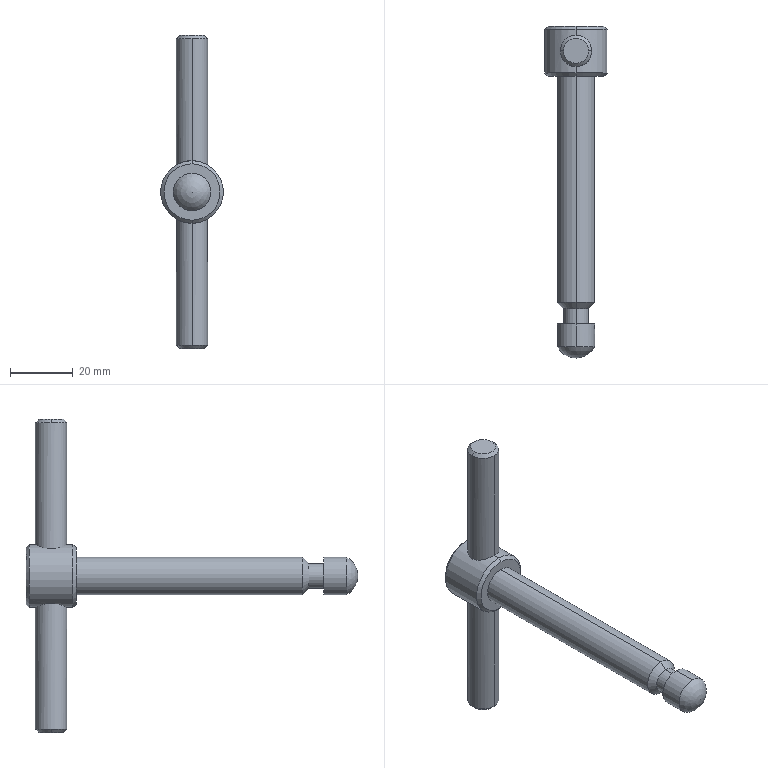Part | SolidWorks | features Revolution 5, Chamfer 4, Dome 3 | 1 solid | 28 faces | box 20 x 106 x 100 mm | volume 20892 mm3 | cylinder 12 | cone 10 | plane 5 | sphere 1 | commonest cylinder face diameters 10 x4 12 x4 7.92 x2 20 x2
STEP:
#1=CARTESIAN_POINT('',(0.,-90.304,-3.96));
#2=VERTEX_POINT('',#1);
#3=CARTESIAN_POINT('',(0.,-90.304,3.96));
#4=VERTEX_POINT('',#3);
#5=CARTESIAN_POINT('',(0.,-90.304,0.));
#6=DIRECTION('',(0.,-1.,0.));
#7=DIRECTION('',(0.,0.,1.));
#8=AXIS2_PLACEMENT_3D('',#5,#6,#7);
#9=CIRCLE('',#8,3.96);
#10=EDGE_CURVE('',#2,#4,#9,.T.);
#11=ORIENTED_EDGE('',*,*,#10,.F.);
#12=CARTESIAN_POINT('',(0.,-88.264,-6.));
#13=VERTEX_POINT('',#12);
#14=CARTESIAN_POINT('',(0.,-88.264,-6.));
#15=DIRECTION('',(0.,0.7071,-0.7071));
#16=VECTOR('',#15,1000.);
#17=LINE('',#14,#16);
#18=EDGE_CURVE('',#2,#13,#17,.T.);
#19=ORIENTED_EDGE('',*,*,#18,.T.);
#20=CARTESIAN_POINT('',(0.,-88.264,6.));
#21=VERTEX_POINT('',#20);
#22=CARTESIAN_POINT('',(0.,-88.264,0.));
#23=DIRECTION('',(0.,1.,0.));
#24=DIRECTION('',(0.,0.,1.));
#25=AXIS2_PLACEMENT_3D('',#22,#23,#24);
#26=CIRCLE('',#25,6.);
#27=EDGE_CURVE('',#21,#13,#26,.T.);
#28=ORIENTED_EDGE('',*,*,#27,.F.);
#29=CARTESIAN_POINT('',(0.,-88.264,6.));
#30=DIRECTION('',(0.,0.7071,0.7071));
#31=VECTOR('',#30,1000.);
#32=LINE('',#29,#31);
#33=EDGE_CURVE('',#4,#21,#32,.T.);
#34=ORIENTED_EDGE('',*,*,#33,.F.);
#35=EDGE_LOOP('',(#11,#19,#28,#34));
#36=FACE_OUTER_BOUND('',#35,.T.);
#37=CARTESIAN_POINT('',(0.,-88.264,0.));
#38=DIRECTION('',(0.,1.,0.));
#39=DIRECTION('',(0.,0.,1.));
#40=AXIS2_PLACEMENT_3D('',#37,#38,#39);
#41=CONICAL_SURFACE('',#40,6.,0.7854);
#42=ADVANCED_FACE('',(#36),#41,.T.);
#43=CARTESIAN_POINT('',(0.,-102.4,6.));
#44=VERTEX_POINT('',#43);
#45=CARTESIAN_POINT('',(0.,-102.4,-6.));
#46=VERTEX_POINT('',#45);
#47=CARTESIAN_POINT('',(0.,-102.4,0.));
#48=DIRECTION('',(0.,1.,0.));
#49=DIRECTION('',(0.,0.,1.));
#50=AXIS2_PLACEMENT_3D('',#47,#48,#49);
#51=CIRCLE('',#50,6.);
#52=EDGE_CURVE('',#44,#46,#51,.T.);
#53=ORIENTED_EDGE('',*,*,#52,.T.);
#54=CARTESIAN_POINT('',(0.,-95.142,-6.));
#55=VERTEX_POINT('',#54);
#56=CARTESIAN_POINT('',(0.,25.503,-6.));
#57=DIRECTION('',(0.,1.,0.));
#58=VECTOR('',#57,1000.);
#59=LINE('',#56,#58);
#60=EDGE_CURVE('',#46,#55,#59,.T.);
#61=ORIENTED_EDGE('',*,*,#60,.T.);
#62=CARTESIAN_POINT('',(0.,-95.142,6.));
#63=VERTEX_POINT('',#62);
#64=CARTESIAN_POINT('',(0.,-95.142,0.));
#65=DIRECTION('',(0.,1.,0.));
#66=DIRECTION('',(0.,0.,1.));
#67=AXIS2_PLACEMENT_3D('',#64,#65,#66);
#68=CIRCLE('',#67,6.);
#69=EDGE_CURVE('',#63,#55,#68,.T.);
#70=ORIENTED_EDGE('',*,*,#69,.F.);
#71=CARTESIAN_POINT('',(0.,25.503,6.));
#72=DIRECTION('',(0.,1.,0.));
#73=VECTOR('',#72,1000.);
#74=LINE('',#71,#73);
#75=EDGE_CURVE('',#44,#63,#74,.T.);
#76=ORIENTED_EDGE('',*,*,#75,.F.);
#77=EDGE_LOOP('',(#53,#61,#70,#76));
#78=FACE_OUTER_BOUND('',#77,.T.);
#79=CARTESIAN_POINT('',(0.,25.503,0.));
#80=DIRECTION('',(0.,1.,0.));
#81=DIRECTION('',(0.,0.,1.));
#82=AXIS2_PLACEMENT_3D('',#79,#80,#81);
#83=CYLINDRICAL_SURFACE('',#82,6.);
#84=ADVANCED_FACE('',(#78),#83,.T.);
#85=CARTESIAN_POINT('',(0.,-95.142,3.96));
#86=VERTEX_POINT('',#85);
#87=CARTESIAN_POINT('',(0.,-95.142,-3.96));
#88=VERTEX_POINT('',#87);
#89=CARTESIAN_POINT('',(0.,-95.142,0.));
#90=DIRECTION('',(0.,1.,0.));
#91=DIRECTION('',(0.,0.,1.));
#92=AXIS2_PLACEMENT_3D('',#89,#90,#91);
#93=CIRCLE('',#92,3.96);
#94=EDGE_CURVE('',#86,#88,#93,.T.);
#95=ORIENTED_EDGE('',*,*,#94,.T.);
#96=CARTESIAN_POINT('',(0.,25.503,-3.96));
#97=DIRECTION('',(0.,1.,0.));
#98=VECTOR('',#97,1000.);
#99=LINE('',#96,#98);
#100=EDGE_CURVE('',#88,#2,#99,.T.);
#101=ORIENTED_EDGE('',*,*,#100,.T.);
#102=ORIENTED_EDGE('',*,*,#10,.T.);
#103=CARTESIAN_POINT('',(0.,25.503,3.96));
#104=DIRECTION('',(0.,1.,0.));
#105=VECTOR('',#104,1000.);
#106=LINE('',#103,#105);
#107=EDGE_CURVE('',#86,#4,#106,.T.);
#108=ORIENTED_EDGE('',*,*,#107,.F.);
#109=EDGE_LOOP('',(#95,#101,#102,#108));
#110=FACE_OUTER_BOUND('',#109,.T.);
#111=CARTESIAN_POINT('',(0.,25.503,0.));
#112=DIRECTION('',(0.,1.,0.));
#113=DIRECTION('',(0.,0.,1.));
#114=AXIS2_PLACEMENT_3D('',#111,#112,#113);
#115=CYLINDRICAL_SURFACE('',#114,3.96);
#116=ADVANCED_FACE('',(#110),#115,.T.);
#117=CARTESIAN_POINT('',(0.,0.,9.));
#118=VERTEX_POINT('',#117);
#119=CARTESIAN_POINT('',(0.,0.,-9.));
#120=VERTEX_POINT('',#119);
#121=CARTESIAN_POINT('',(0.,0.,0.));
#122=DIRECTION('',(0.,1.,0.));
#123=DIRECTION('',(0.,0.,-1.));
#124=AXIS2_PLACEMENT_3D('',#121,#122,#123);
#125=CIRCLE('',#124,9.);
#126=EDGE_CURVE('',#118,#120,#125,.T.);
#127=ORIENTED_EDGE('',*,*,#126,.F.);
#128=CARTESIAN_POINT('',(0.,-1.,10.));
#129=VERTEX_POINT('',#128);
#130=CARTESIAN_POINT('',(0.,0.,9.));
#131=DIRECTION('',(0.,-0.7071,0.7071));
#132=VECTOR('',#131,1000.);
#133=LINE('',#130,#132);
#134=EDGE_CURVE('',#118,#129,#133,.T.);
#135=ORIENTED_EDGE('',*,*,#134,.T.);
#136=CARTESIAN_POINT('',(0.,-1.,-10.));
#137=VERTEX_POINT('',#136);
#138=CARTESIAN_POINT('',(0.,-1.,0.));
#139=DIRECTION('',(0.,-1.,0.));
#140=DIRECTION('',(0.,0.,-1.));
#141=AXIS2_PLACEMENT_3D('',#138,#139,#140);
#142=CIRCLE('',#141,10.);
#143=EDGE_CURVE('',#137,#129,#142,.T.);
#144=ORIENTED_EDGE('',*,*,#143,.F.);
#145=CARTESIAN_POINT('',(0.,0.,-9.));
#146=DIRECTION('',(0.,-0.7071,-0.7071));
#147=VECTOR('',#146,1000.);
#148=LINE('',#145,#147);
#149=EDGE_CURVE('',#120,#137,#148,.T.);
#150=ORIENTED_EDGE('',*,*,#149,.F.);
#151=EDGE_LOOP('',(#127,#135,#144,#150));
#152=FACE_OUTER_BOUND('',#151,.T.);
#153=CARTESIAN_POINT('',(0.,0.,0.));
#154=DIRECTION('',(0.,-1.,0.));
#155=DIRECTION('',(0.,0.,-1.));
#156=AXIS2_PLACEMENT_3D('',#153,#154,#155);
#157=CONICAL_SURFACE('',#156,9.,0.7854);
#158=ADVANCED_FACE('',(#152),#157,.T.);
#159=CARTESIAN_POINT('',(0.,-16.,-9.));
#160=VERTEX_POINT('',#159);
#161=CARTESIAN_POINT('',(0.,-16.,9.));
#162=VERTEX_POINT('',#161);
#163=CARTESIAN_POINT('',(0.,-16.,0.));
#164=DIRECTION('',(0.,-1.,0.));
#165=DIRECTION('',(0.,0.,1.));
#166=AXIS2_PLACEMENT_3D('',#163,#164,#165);
#167=CIRCLE('',#166,9.);
#168=EDGE_CURVE('',#160,#162,#167,.T.);
#169=ORIENTED_EDGE('',*,*,#168,.F.);
#170=CARTESIAN_POINT('',(0.,-15.,-10.));
#171=VERTEX_POINT('',#170);
#172=CARTESIAN_POINT('',(0.,-15.,-10.));
#173=DIRECTION('',(0.,0.7071,-0.7071));
#174=VECTOR('',#173,1000.);
#175=LINE('',#172,#174);
#176=EDGE_CURVE('',#160,#171,#175,.T.);
#177=ORIENTED_EDGE('',*,*,#176,.T.);
#178=CARTESIAN_POINT('',(0.,-15.,10.));
#179=VERTEX_POINT('',#178);
#180=CARTESIAN_POINT('',(0.,-15.,0.));
#181=DIRECTION('',(0.,1.,0.));
#182=DIRECTION('',(0.,0.,1.));
#183=AXIS2_PLACEMENT_3D('',#180,#181,#182);
#184=CIRCLE('',#183,10.);
#185=EDGE_CURVE('',#179,#171,#184,.T.);
#186=ORIENTED_EDGE('',*,*,#185,.F.);
#187=CARTESIAN_POINT('',(0.,-15.,10.));
#188=DIRECTION('',(0.,0.7071,0.7071));
#189=VECTOR('',#188,1000.);
#190=LINE('',#187,#189);
#191=EDGE_CURVE('',#162,#179,#190,.T.);
#192=ORIENTED_EDGE('',*,*,#191,.F.);
#193=EDGE_LOOP('',(#169,#177,#186,#192));
#194=FACE_OUTER_BOUND('',#193,.T.);
#195=CARTESIAN_POINT('',(0.,-15.,0.));
#196=DIRECTION('',(0.,1.,0.));
#197=DIRECTION('',(0.,0.,1.));
#198=AXIS2_PLACEMENT_3D('',#195,#196,#197);
#199=CONICAL_SURFACE('',#198,10.,0.7854);
#200=ADVANCED_FACE('',(#194),#199,.T.);
#201=CARTESIAN_POINT('',(4.,-8.,50.));
#202=VERTEX_POINT('',#201);
#203=CARTESIAN_POINT('',(-4.,-8.,50.));
#204=VERTEX_POINT('',#203);
#205=CARTESIAN_POINT('',(0.,-8.,50.));
#206=DIRECTION('',(0.,0.,1.));
#207=DIRECTION('',(0.,-1.,0.));
#208=AXIS2_PLACEMENT_3D('',#205,#206,#207);
#209=CIRCLE('',#208,4.);
#210=EDGE_CURVE('',#202,#204,#209,.T.);
#211=ORIENTED_EDGE('',*,*,#210,.F.);
#212=CARTESIAN_POINT('',(5.,-8.,49.));
#213=VERTEX_POINT('',#212);
#214=CARTESIAN_POINT('',(5.,-8.,49.));
#215=DIRECTION('',(0.7071,0.,-0.7071));
#216=VECTOR('',#215,1000.);
#217=LINE('',#214,#216);
#218=EDGE_CURVE('',#202,#213,#217,.T.);
#219=ORIENTED_EDGE('',*,*,#218,.T.);
#220=CARTESIAN_POINT('',(0.,-3.,49.));
#221=VERTEX_POINT('',#220);
#222=CARTESIAN_POINT('',(0.,-8.,49.));
#223=DIRECTION('',(0.,0.,-1.));
#224=DIRECTION('',(1.,0.,0.));
#225=AXIS2_PLACEMENT_3D('',#222,#223,#224);
#226=CIRCLE('',#225,5.);
#227=EDGE_CURVE('',#221,#213,#226,.T.);
#228=ORIENTED_EDGE('',*,*,#227,.F.);
#229=CARTESIAN_POINT('',(-5.,-8.,49.));
#230=VERTEX_POINT('',#229);
#231=CARTESIAN_POINT('',(0.,-8.,49.));
#232=DIRECTION('',(0.,0.,-1.));
#233=DIRECTION('',(1.,0.,0.));
#234=AXIS2_PLACEMENT_3D('',#231,#232,#233);
#235=CIRCLE('',#234,5.);
#236=EDGE_CURVE('',#230,#221,#235,.T.);
#237=ORIENTED_EDGE('',*,*,#236,.F.);
#238=CARTESIAN_POINT('',(-5.,-8.,49.));
#239=DIRECTION('',(-0.7071,0.,-0.7071));
#240=VECTOR('',#239,1000.);
#241=LINE('',#238,#240);
#242=EDGE_CURVE('',#204,#230,#241,.T.);
#243=ORIENTED_EDGE('',*,*,#242,.F.);
#244=EDGE_LOOP('',(#211,#219,#228,#237,#243));
#245=FACE_OUTER_BOUND('',#244,.T.);
#246=CARTESIAN_POINT('',(0.,-8.,49.));
#247=DIRECTION('',(0.,0.,-1.));
#248=DIRECTION('',(-1.,0.,0.));
#249=AXIS2_PLACEMENT_3D('',#246,#247,#248);
#250=CONICAL_SURFACE('',#249,5.,0.7854);
#251=ADVANCED_FACE('',(#245),#250,.T.);
#252=CARTESIAN_POINT('',(-4.,-8.,-50.));
#253=VERTEX_POINT('',#252);
#254=CARTESIAN_POINT('',(4.,-8.,-50.));
#255=VERTEX_POINT('',#254);
#256=CARTESIAN_POINT('',(0.,-8.,-50.));
#257=DIRECTION('',(0.,0.,-1.));
#258=DIRECTION('',(0.,1.,0.));
#259=AXIS2_PLACEMENT_3D('',#256,#257,#258);
#260=CIRCLE('',#259,4.);
#261=EDGE_CURVE('',#253,#255,#260,.T.);
#262=ORIENTED_EDGE('',*,*,#261,.F.);
#263=CARTESIAN_POINT('',(-5.,-8.,-49.));
#264=VERTEX_POINT('',#263);
#265=CARTESIAN_POINT('',(-4.,-8.,-50.));
#266=DIRECTION('',(-0.7071,0.,0.7071));
#267=VECTOR('',#266,1000.);
#268=LINE('',#265,#267);
#269=EDGE_CURVE('',#253,#264,#268,.T.);
#270=ORIENTED_EDGE('',*,*,#269,.T.);
#271=CARTESIAN_POINT('',(0.,-3.,-49.));
#272=VERTEX_POINT('',#271);
#273=CARTESIAN_POINT('',(0.,-8.,-49.));
#274=DIRECTION('',(0.,0.,1.));
#275=DIRECTION('',(-1.,0.,0.));
#276=AXIS2_PLACEMENT_3D('',#273,#274,#275);
#277=CIRCLE('',#276,5.);
#278=EDGE_CURVE('',#272,#264,#277,.T.);
#279=ORIENTED_EDGE('',*,*,#278,.F.);
#280=CARTESIAN_POINT('',(5.,-8.,-49.));
#281=VERTEX_POINT('',#280);
#282=CARTESIAN_POINT('',(0.,-8.,-49.));
#283=DIRECTION('',(0.,0.,1.));
#284=DIRECTION('',(-1.,0.,0.));
#285=AXIS2_PLACEMENT_3D('',#282,#283,#284);
#286=CIRCLE('',#285,5.);
#287=EDGE_CURVE('',#281,#272,#286,.T.);
#288=ORIENTED_EDGE('',*,*,#287,.F.);
#289=CARTESIAN_POINT('',(4.,-8.,-50.));
#290=DIRECTION('',(0.7071,0.,0.7071));
#291=VECTOR('',#290,1000.);
#292=LINE('',#289,#291);
#293=EDGE_CURVE('',#255,#281,#292,.T.);
#294=ORIENTED_EDGE('',*,*,#293,.F.);
#295=EDGE_LOOP('',(#262,#270,#279,#288,#294));
#296=FACE_OUTER_BOUND('',#295,.T.);
#297=CARTESIAN_POINT('',(0.,-8.,-50.));
#298=DIRECTION('',(0.,0.,1.));
#299=DIRECTION('',(1.,0.,0.));
#300=AXIS2_PLACEMENT_3D('',#297,#298,#299);
#301=CONICAL_SURFACE('',#300,4.,0.7854);
#302=ADVANCED_FACE('',(#296),#301,.T.);
#303=ORIENTED_EDGE('',*,*,#227,.T.);
#304=CARTESIAN_POINT('',(0.,-13.,49.));
#305=VERTEX_POINT('',#304);
#306=CARTESIAN_POINT('',(0.,-8.,49.));
#307=DIRECTION('',(0.,0.,-1.));
#308=DIRECTION('',(1.,0.,0.));
#309=AXIS2_PLACEMENT_3D('',#306,#307,#308);
#310=CIRCLE('',#309,5.);
#311=EDGE_CURVE('',#213,#305,#310,.T.);
#312=ORIENTED_EDGE('',*,*,#311,.T.);
#313=CARTESIAN_POINT('',(0.,-13.,10.));
#314=VERTEX_POINT('',#313);
#315=CARTESIAN_POINT('',(0.,-13.,-27.254));
#316=DIRECTION('',(0.,0.,-1.));
#317=VECTOR('',#316,1000.);
#318=LINE('',#315,#317);
#319=EDGE_CURVE('',#305,#314,#318,.T.);
#320=ORIENTED_EDGE('',*,*,#319,.T.);
#321=CARTESIAN_POINT('',(0.,-3.,10.));
#322=VERTEX_POINT('',#321);
#323=CARTESIAN_POINT('',(0.,-3.,10.));
#324=CARTESIAN_POINT('',(0.3314,-3.,10.));
#325=CARTESIAN_POINT('',(0.6687,-3.034,9.983));
#326=CARTESIAN_POINT('',(1.317,-3.165,9.918));
#327=CARTESIAN_POINT('',(1.631,-3.262,9.871));
#328=CARTESIAN_POINT('',(2.24,-3.518,9.751));
#329=CARTESIAN_POINT('',(2.526,-3.673,9.68));
#330=CARTESIAN_POINT('',(3.061,-4.034,9.524));
#331=CARTESIAN_POINT('',(3.314,-4.242,9.438));
#332=CARTESIAN_POINT('',(3.767,-4.697,9.266));
#333=CARTESIAN_POINT('',(3.971,-4.944,9.18));
#334=CARTESIAN_POINT('',(4.331,-5.48,9.016));
#335=CARTESIAN_POINT('',(4.487,-5.769,8.938));
#336=CARTESIAN_POINT('',(4.737,-6.367,8.808));
#337=CARTESIAN_POINT('',(4.834,-6.679,8.754));
#338=CARTESIAN_POINT('',(4.933,-7.168,8.699));
#339=CARTESIAN_POINT('',(4.958,-7.334,8.684));
#340=CARTESIAN_POINT('',(4.991,-7.664,8.665));
#341=CARTESIAN_POINT('',(5.008,-7.994,8.656));
#342=CARTESIAN_POINT('',(4.992,-8.325,8.665));
#343=CARTESIAN_POINT('',(4.959,-8.657,8.684));
#344=CARTESIAN_POINT('',(4.935,-8.823,8.698));
#345=CARTESIAN_POINT('',(4.836,-9.311,8.753));
#346=CARTESIAN_POINT('',(4.74,-9.625,8.806));
#347=CARTESIAN_POINT('',(4.487,-10.23,8.938));
#348=CARTESIAN_POINT('',(4.332,-10.518,9.015));
#349=CARTESIAN_POINT('',(3.973,-11.053,9.179));
#350=CARTESIAN_POINT('',(3.767,-11.304,9.267));
#351=CARTESIAN_POINT('',(3.311,-11.761,9.439));
#352=CARTESIAN_POINT('',(3.064,-11.965,9.523));
#353=CARTESIAN_POINT('',(2.528,-12.326,9.679));
#354=CARTESIAN_POINT('',(2.237,-12.483,9.751));
#355=CARTESIAN_POINT('',(1.635,-12.736,9.87));
#356=CARTESIAN_POINT('',(1.323,-12.833,9.918));
#357=CARTESIAN_POINT('',(0.6735,-12.965,9.983));
#358=CARTESIAN_POINT('',(0.3359,-13.,10.));
#359=CARTESIAN_POINT('',(0.,-13.,10.));
#360=B_SPLINE_CURVE_WITH_KNOTS('',3,(#323,#324,#325,#326,#327,#328,#329,#330,#331,#332,#333,#334,#335,#336,#337,#338,#339,#340,#341,#342,#343,#344,#345,#346,#347,#348,#349,#350,#351,#352,#353,#354,#355,#356,#357,#358,#359),.UNSPECIFIED.,.F.,.F.,(4,2,2,2,2,2,2,2,2,1,2,2,2,2,2,2,2,2,4),(0.0159,0.0169,0.01789,0.01888,0.01987,0.02087,0.02186,0.02285,0.02335,0.02384,0.02434,0.02484,0.02583,0.02682,0.02781,0.02881,0.0298,0.03079,0.03178),.UNSPECIFIED.);
#361=EDGE_CURVE('',#322,#314,#360,.T.);
#362=ORIENTED_EDGE('',*,*,#361,.F.);
#363=CARTESIAN_POINT('',(0.,-3.,-27.254));
#364=DIRECTION('',(0.,0.,-1.));
#365=VECTOR('',#364,1000.);
#366=LINE('',#363,#365);
#367=EDGE_CURVE('',#221,#322,#366,.T.);
#368=ORIENTED_EDGE('',*,*,#367,.F.);
#369=EDGE_LOOP('',(#303,#312,#320,#362,#368));
#370=FACE_OUTER_BOUND('',#369,.T.);
#371=CARTESIAN_POINT('',(0.,-8.,-27.254));
#372=DIRECTION('',(0.,0.,-1.));
#373=DIRECTION('',(0.,1.,0.));
#374=AXIS2_PLACEMENT_3D('',#371,#372,#373);
#375=CYLINDRICAL_SURFACE('',#374,5.);
#376=ADVANCED_FACE('',(#370),#375,.T.);
#377=CARTESIAN_POINT('',(0.,-13.,-10.));
#378=VERTEX_POINT('',#377);
#379=CARTESIAN_POINT('',(0.,-3.,-10.));
#380=VERTEX_POINT('',#379);
#381=CARTESIAN_POINT('',(0.,-13.,-10.));
#382=CARTESIAN_POINT('',(0.3314,-13.,-10.));
#383=CARTESIAN_POINT('',(0.6687,-12.966,-9.983));
#384=CARTESIAN_POINT('',(1.317,-12.835,-9.918));
#385=CARTESIAN_POINT('',(1.631,-12.738,-9.871));
#386=CARTESIAN_POINT('',(2.24,-12.482,-9.751));
#387=CARTESIAN_POINT('',(2.526,-12.327,-9.68));
#388=CARTESIAN_POINT('',(3.061,-11.966,-9.524));
#389=CARTESIAN_POINT('',(3.314,-11.758,-9.438));
#390=CARTESIAN_POINT('',(3.767,-11.303,-9.266));
#391=CARTESIAN_POINT('',(3.971,-11.056,-9.18));
#392=CARTESIAN_POINT('',(4.331,-10.52,-9.016));
#393=CARTESIAN_POINT('',(4.487,-10.231,-8.938));
#394=CARTESIAN_POINT('',(4.737,-9.633,-8.808));
#395=CARTESIAN_POINT('',(4.834,-9.321,-8.754));
#396=CARTESIAN_POINT('',(4.933,-8.832,-8.699));
#397=CARTESIAN_POINT('',(4.958,-8.666,-8.684));
#398=CARTESIAN_POINT('',(4.991,-8.336,-8.665));
#399=CARTESIAN_POINT('',(5.008,-8.006,-8.656));
#400=CARTESIAN_POINT('',(4.992,-7.675,-8.665));
#401=CARTESIAN_POINT('',(4.959,-7.343,-8.684));
#402=CARTESIAN_POINT('',(4.935,-7.177,-8.698));
#403=CARTESIAN_POINT('',(4.836,-6.689,-8.753));
#404=CARTESIAN_POINT('',(4.74,-6.375,-8.806));
#405=CARTESIAN_POINT('',(4.487,-5.77,-8.938));
#406=CARTESIAN_POINT('',(4.332,-5.482,-9.015));
#407=CARTESIAN_POINT('',(3.973,-4.947,-9.179));
#408=CARTESIAN_POINT('',(3.767,-4.696,-9.267));
#409=CARTESIAN_POINT('',(3.311,-4.239,-9.439));
#410=CARTESIAN_POINT('',(3.064,-4.035,-9.523));
#411=CARTESIAN_POINT('',(2.528,-3.674,-9.679));
#412=CARTESIAN_POINT('',(2.237,-3.517,-9.751));
#413=CARTESIAN_POINT('',(1.635,-3.264,-9.87));
#414=CARTESIAN_POINT('',(1.323,-3.167,-9.918));
#415=CARTESIAN_POINT('',(0.6735,-3.035,-9.983));
#416=CARTESIAN_POINT('',(0.3359,-3.,-10.));
#417=CARTESIAN_POINT('',(0.,-3.,-10.));
#418=B_SPLINE_CURVE_WITH_KNOTS('',3,(#381,#382,#383,#384,#385,#386,#387,#388,#389,#390,#391,#392,#393,#394,#395,#396,#397,#398,#399,#400,#401,#402,#403,#404,#405,#406,#407,#408,#409,#410,#411,#412,#413,#414,#415,#416,#417),.UNSPECIFIED.,.F.,.F.,(4,2,2,2,2,2,2,2,2,1,2,2,2,2,2,2,2,2,4),(0.0159,0.0169,0.01789,0.01888,0.01987,0.02087,0.02186,0.02285,0.02335,0.02384,0.02434,0.02484,0.02583,0.02682,0.02781,0.02881,0.0298,0.03079,0.03178),.UNSPECIFIED.);
#419=EDGE_CURVE('',#378,#380,#418,.T.);
#420=ORIENTED_EDGE('',*,*,#419,.F.);
#421=CARTESIAN_POINT('',(0.,-13.,-49.));
#422=VERTEX_POINT('',#421);
#423=CARTESIAN_POINT('',(0.,-13.,-27.254));
#424=DIRECTION('',(0.,0.,-1.));
#425=VECTOR('',#424,1000.);
#426=LINE('',#423,#425);
#427=EDGE_CURVE('',#378,#422,#426,.T.);
#428=ORIENTED_EDGE('',*,*,#427,.T.);
#429=CARTESIAN_POINT('',(0.,-8.,-49.));
#430=DIRECTION('',(0.,0.,1.));
#431=DIRECTION('',(-1.,0.,0.));
#432=AXIS2_PLACEMENT_3D('',#429,#430,#431);
#433=CIRCLE('',#432,5.);
#434=EDGE_CURVE('',#422,#281,#433,.T.);
#435=ORIENTED_EDGE('',*,*,#434,.T.);
#436=ORIENTED_EDGE('',*,*,#287,.T.);
#437=CARTESIAN_POINT('',(0.,-3.,-27.254));
#438=DIRECTION('',(0.,0.,-1.));
#439=VECTOR('',#438,1000.);
#440=LINE('',#437,#439);
#441=EDGE_CURVE('',#380,#272,#440,.T.);
#442=ORIENTED_EDGE('',*,*,#441,.F.);
#443=EDGE_LOOP('',(#420,#428,#435,#436,#442));
#444=FACE_OUTER_BOUND('',#443,.T.);
#445=CARTESIAN_POINT('',(0.,-8.,-27.254));
#446=DIRECTION('',(0.,0.,-1.));
#447=DIRECTION('',(0.,1.,0.));
#448=AXIS2_PLACEMENT_3D('',#445,#446,#447);
#449=CYLINDRICAL_SURFACE('',#448,5.);
#450=ADVANCED_FACE('',(#444),#449,.T.);
#451=ORIENTED_EDGE('',*,*,#27,.T.);
#452=CARTESIAN_POINT('',(0.,-16.,-6.));
#453=VERTEX_POINT('',#452);
#454=CARTESIAN_POINT('',(0.,25.503,-6.));
#455=DIRECTION('',(0.,1.,0.));
#456=VECTOR('',#455,1000.);
#457=LINE('',#454,#456);
#458=EDGE_CURVE('',#13,#453,#457,.T.);
#459=ORIENTED_EDGE('',*,*,#458,.T.);
#460=CARTESIAN_POINT('',(0.,-16.,6.));
#461=VERTEX_POINT('',#460);
#462=CARTESIAN_POINT('',(0.,-16.,0.));
#463=DIRECTION('',(0.,1.,0.));
#464=DIRECTION('',(0.,0.,1.));
#465=AXIS2_PLACEMENT_3D('',#462,#463,#464);
#466=CIRCLE('',#465,6.);
#467=EDGE_CURVE('',#461,#453,#466,.T.);
#468=ORIENTED_EDGE('',*,*,#467,.F.);
#469=CARTESIAN_POINT('',(0.,25.503,6.));
#470=DIRECTION('',(0.,1.,0.));
#471=VECTOR('',#470,1000.);
#472=LINE('',#469,#471);
#473=EDGE_CURVE('',#21,#461,#472,.T.);
#474=ORIENTED_EDGE('',*,*,#473,.F.);
#475=EDGE_LOOP('',(#451,#459,#468,#474));
#476=FACE_OUTER_BOUND('',#475,.T.);
#477=CARTESIAN_POINT('',(0.,25.503,0.));
#478=DIRECTION('',(0.,1.,0.));
#479=DIRECTION('',(0.,0.,1.));
#480=AXIS2_PLACEMENT_3D('',#477,#478,#479);
#481=CYLINDRICAL_SURFACE('',#480,6.);
#482=ADVANCED_FACE('',(#476),#481,.T.);
#483=ORIENTED_EDGE('',*,*,#185,.T.);
#484=CARTESIAN_POINT('',(0.,25.503,-10.));
#485=DIRECTION('',(0.,1.,0.));
#486=VECTOR('',#485,1000.);
#487=LINE('',#484,#486);
#488=EDGE_CURVE('',#171,#378,#487,.T.);
#489=ORIENTED_EDGE('',*,*,#488,.T.);
#490=ORIENTED_EDGE('',*,*,#419,.T.);
#491=CARTESIAN_POINT('',(0.,25.503,-10.));
#492=DIRECTION('',(0.,1.,0.));
#493=VECTOR('',#492,1000.);
#494=LINE('',#491,#493);
#495=EDGE_CURVE('',#380,#137,#494,.T.);
#496=ORIENTED_EDGE('',*,*,#495,.T.);
#497=ORIENTED_EDGE('',*,*,#143,.T.);
#498=CARTESIAN_POINT('',(0.,25.503,10.));
#499=DIRECTION('',(0.,1.,0.));
#500=VECTOR('',#499,1000.);
#501=LINE('',#498,#500);
#502=EDGE_CURVE('',#322,#129,#501,.T.);
#503=ORIENTED_EDGE('',*,*,#502,.F.);
#504=ORIENTED_EDGE('',*,*,#361,.T.);
#505=CARTESIAN_POINT('',(0.,25.503,10.));
#506=DIRECTION('',(0.,1.,0.));
#507=VECTOR('',#506,1000.);
#508=LINE('',#505,#507);
#509=EDGE_CURVE('',#179,#314,#508,.T.);
#510=ORIENTED_EDGE('',*,*,#509,.F.);
#511=EDGE_LOOP('',(#483,#489,#490,#496,#497,#503,#504,#510));
#512=FACE_OUTER_BOUND('',#511,.T.);
#513=CARTESIAN_POINT('',(0.,25.503,0.));
#514=DIRECTION('',(0.,1.,0.));
#515=DIRECTION('',(0.,0.,1.));
#516=AXIS2_PLACEMENT_3D('',#513,#514,#515);
#517=CYLINDRICAL_SURFACE('',#516,10.);
#518=ADVANCED_FACE('',(#512),#517,.T.);
#519=CARTESIAN_POINT('',(0.,0.,0.));
#520=DIRECTION('',(0.,1.,0.));
#521=DIRECTION('',(0.,0.,-1.));
#522=AXIS2_PLACEMENT_3D('',#519,#520,#521);
#523=CIRCLE('',#522,9.);
#524=EDGE_CURVE('',#120,#118,#523,.T.);
#525=ORIENTED_EDGE('',*,*,#524,.T.);
#526=ORIENTED_EDGE('',*,*,#126,.T.);
#527=EDGE_LOOP('',(#525,#526));
#528=FACE_OUTER_BOUND('',#527,.T.);
#529=CARTESIAN_POINT('',(0.,0.,0.));
#530=DIRECTION('',(0.,-1.,0.));
#531=DIRECTION('',(0.,0.,-1.));
#532=AXIS2_PLACEMENT_3D('',#529,#530,#531);
#533=PLANE('',#532);
#534=ADVANCED_FACE('',(#528),#533,.F.);
#535=ORIENTED_EDGE('',*,*,#488,.F.);
#536=CARTESIAN_POINT('',(0.,-15.,0.));
#537=DIRECTION('',(0.,1.,0.));
#538=DIRECTION('',(0.,0.,1.));
#539=AXIS2_PLACEMENT_3D('',#536,#537,#538);
#540=CIRCLE('',#539,10.);
#541=EDGE_CURVE('',#171,#179,#540,.T.);
#542=ORIENTED_EDGE('',*,*,#541,.T.);
#543=ORIENTED_EDGE('',*,*,#509,.T.);
#544=CARTESIAN_POINT('',(0.,-13.,10.));
#545=CARTESIAN_POINT('',(-0.3365,-13.,10.));
#546=CARTESIAN_POINT('',(-0.6663,-12.966,9.983));
#547=CARTESIAN_POINT('',(-1.314,-12.836,9.919));
#548=CARTESIAN_POINT('',(-1.634,-12.737,9.87));
#549=CARTESIAN_POINT('',(-2.238,-12.483,9.751));
#550=CARTESIAN_POINT('',(-2.523,-12.329,9.68));
#551=CARTESIAN_POINT('',(-3.063,-11.965,9.524));
#552=CARTESIAN_POINT('',(-3.313,-11.758,9.438));
#553=CARTESIAN_POINT('',(-3.766,-11.305,9.267));
#554=CARTESIAN_POINT('',(-3.972,-11.054,9.179));
#555=CARTESIAN_POINT('',(-4.333,-10.516,9.015));
#556=CARTESIAN_POINT('',(-4.486,-10.232,8.939));
#557=CARTESIAN_POINT('',(-4.674,-9.783,8.841));
#558=CARTESIAN_POINT('',(-4.73,-9.629,8.811));
#559=CARTESIAN_POINT('',(-4.827,-9.313,8.758));
#560=CARTESIAN_POINT('',(-4.868,-9.152,8.735));
#561=CARTESIAN_POINT('',(-4.966,-8.666,8.68));
#562=CARTESIAN_POINT('',(-5.,-8.338,8.66));
#563=CARTESIAN_POINT('',(-5.,-7.838,8.66));
#564=CARTESIAN_POINT('',(-4.992,-7.67,8.665));
#565=CARTESIAN_POINT('',(-4.959,-7.337,8.684));
#566=CARTESIAN_POINT('',(-4.934,-7.173,8.698));
#567=CARTESIAN_POINT('',(-4.836,-6.688,8.753));
#568=CARTESIAN_POINT('',(-4.738,-6.37,8.807));
#569=CARTESIAN_POINT('',(-4.485,-5.765,8.939));
#570=CARTESIAN_POINT('',(-4.331,-5.48,9.016));
#571=CARTESIAN_POINT('',(-3.97,-4.943,9.18));
#572=CARTESIAN_POINT('',(-3.763,-4.692,9.268));
#573=CARTESIAN_POINT('',(-3.309,-4.238,9.44));
#574=CARTESIAN_POINT('',(-3.061,-4.033,9.524));
#575=CARTESIAN_POINT('',(-2.52,-3.669,9.681));
#576=CARTESIAN_POINT('',(-2.233,-3.514,9.752));
#577=CARTESIAN_POINT('',(-1.783,-3.326,9.841));
#578=CARTESIAN_POINT('',(-1.629,-3.27,9.868));
#579=CARTESIAN_POINT('',(-1.314,-3.173,9.915));
#580=CARTESIAN_POINT('',(-1.152,-3.132,9.935));
#581=CARTESIAN_POINT('',(-0.6614,-3.033,9.984));
#582=CARTESIAN_POINT('',(-0.332,-3.,10.));
#583=CARTESIAN_POINT('',(0.,-3.,10.));
#584=B_SPLINE_CURVE_WITH_KNOTS('',3,(#544,#545,#546,#547,#548,#549,#550,#551,#552,#553,#554,#555,#556,#557,#558,#559,#560,#561,#562,#563,#564,#565,#566,#567,#568,#569,#570,#571,#572,#573,#574,#575,#576,#577,#578,#579,#580,#581,#582,#583),.UNSPECIFIED.,.F.,.F.,(4,2,2,2,2,2,2,2,2,2,2,2,2,2,2,2,2,2,2,4),(0.,0.0009941,0.001988,0.002982,0.003976,0.00497,0.005964,0.006461,0.006958,0.007952,0.008449,0.008947,0.009941,0.01093,0.01193,0.01292,0.01392,0.01441,0.01491,0.0159),.UNSPECIFIED.);
#585=EDGE_CURVE('',#314,#322,#584,.T.);
#586=ORIENTED_EDGE('',*,*,#585,.T.);
#587=ORIENTED_EDGE('',*,*,#502,.T.);
#588=CARTESIAN_POINT('',(0.,-1.,0.));
#589=DIRECTION('',(0.,-1.,0.));
#590=DIRECTION('',(0.,0.,-1.));
#591=AXIS2_PLACEMENT_3D('',#588,#589,#590);
#592=CIRCLE('',#591,10.);
#593=EDGE_CURVE('',#129,#137,#592,.T.);
#594=ORIENTED_EDGE('',*,*,#593,.T.);
#595=ORIENTED_EDGE('',*,*,#495,.F.);
#596=CARTESIAN_POINT('',(0.,-3.,-10.));
#597=CARTESIAN_POINT('',(-0.3365,-3.,-10.));
#598=CARTESIAN_POINT('',(-0.6663,-3.034,-9.983));
#599=CARTESIAN_POINT('',(-1.314,-3.164,-9.919));
#600=CARTESIAN_POINT('',(-1.634,-3.263,-9.87));
#601=CARTESIAN_POINT('',(-2.238,-3.517,-9.751));
#602=CARTESIAN_POINT('',(-2.523,-3.671,-9.68));
#603=CARTESIAN_POINT('',(-3.063,-4.035,-9.524));
#604=CARTESIAN_POINT('',(-3.313,-4.242,-9.438));
#605=CARTESIAN_POINT('',(-3.766,-4.695,-9.267));
#606=CARTESIAN_POINT('',(-3.972,-4.946,-9.179));
#607=CARTESIAN_POINT('',(-4.333,-5.484,-9.015));
#608=CARTESIAN_POINT('',(-4.486,-5.768,-8.939));
#609=CARTESIAN_POINT('',(-4.674,-6.217,-8.841));
#610=CARTESIAN_POINT('',(-4.73,-6.371,-8.811));
#611=CARTESIAN_POINT('',(-4.827,-6.687,-8.758));
#612=CARTESIAN_POINT('',(-4.868,-6.848,-8.735));
#613=CARTESIAN_POINT('',(-4.966,-7.334,-8.68));
#614=CARTESIAN_POINT('',(-5.,-7.662,-8.66));
#615=CARTESIAN_POINT('',(-5.,-8.162,-8.66));
#616=CARTESIAN_POINT('',(-4.992,-8.33,-8.665));
#617=CARTESIAN_POINT('',(-4.959,-8.663,-8.684));
#618=CARTESIAN_POINT('',(-4.934,-8.827,-8.698));
#619=CARTESIAN_POINT('',(-4.836,-9.312,-8.753));
#620=CARTESIAN_POINT('',(-4.738,-9.63,-8.807));
#621=CARTESIAN_POINT('',(-4.485,-10.235,-8.939));
#622=CARTESIAN_POINT('',(-4.331,-10.52,-9.016));
#623=CARTESIAN_POINT('',(-3.97,-11.057,-9.18));
#624=CARTESIAN_POINT('',(-3.763,-11.308,-9.268));
#625=CARTESIAN_POINT('',(-3.309,-11.762,-9.44));
#626=CARTESIAN_POINT('',(-3.061,-11.967,-9.524));
#627=CARTESIAN_POINT('',(-2.52,-12.331,-9.681));
#628=CARTESIAN_POINT('',(-2.233,-12.486,-9.752));
#629=CARTESIAN_POINT('',(-1.783,-12.674,-9.841));
#630=CARTESIAN_POINT('',(-1.629,-12.73,-9.868));
#631=CARTESIAN_POINT('',(-1.314,-12.827,-9.915));
#632=CARTESIAN_POINT('',(-1.152,-12.868,-9.935));
#633=CARTESIAN_POINT('',(-0.6614,-12.967,-9.984));
#634=CARTESIAN_POINT('',(-0.332,-13.,-10.));
#635=CARTESIAN_POINT('',(0.,-13.,-10.));
#636=B_SPLINE_CURVE_WITH_KNOTS('',3,(#596,#597,#598,#599,#600,#601,#602,#603,#604,#605,#606,#607,#608,#609,#610,#611,#612,#613,#614,#615,#616,#617,#618,#619,#620,#621,#622,#623,#624,#625,#626,#627,#628,#629,#630,#631,#632,#633,#634,#635),.UNSPECIFIED.,.F.,.F.,(4,2,2,2,2,2,2,2,2,2,2,2,2,2,2,2,2,2,2,4),(0.,0.0009941,0.001988,0.002982,0.003976,0.00497,0.005964,0.006461,0.006958,0.007952,0.008449,0.008947,0.009941,0.01093,0.01193,0.01292,0.01392,0.01441,0.01491,0.0159),.UNSPECIFIED.);
#637=EDGE_CURVE('',#380,#378,#636,.T.);
#638=ORIENTED_EDGE('',*,*,#637,.T.);
#639=EDGE_LOOP('',(#535,#542,#543,#586,#587,#594,#595,#638));
#640=FACE_OUTER_BOUND('',#639,.T.);
#641=CARTESIAN_POINT('',(0.,25.503,0.));
#642=DIRECTION('',(0.,1.,0.));
#643=DIRECTION('',(0.,0.,1.));
#644=AXIS2_PLACEMENT_3D('',#641,#642,#643);
#645=CYLINDRICAL_SURFACE('',#644,10.);
#646=ADVANCED_FACE('',(#640),#645,.T.);
#647=CARTESIAN_POINT('',(0.,-16.,0.));
#648=DIRECTION('',(0.,-1.,0.));
#649=DIRECTION('',(0.,0.,1.));
#650=AXIS2_PLACEMENT_3D('',#647,#648,#649);
#651=CIRCLE('',#650,9.);
#652=EDGE_CURVE('',#162,#160,#651,.T.);
#653=ORIENTED_EDGE('',*,*,#652,.T.);
#654=ORIENTED_EDGE('',*,*,#168,.T.);
#655=EDGE_LOOP('',(#653,#654));
#656=FACE_OUTER_BOUND('',#655,.T.);
#657=ORIENTED_EDGE('',*,*,#467,.T.);
#658=CARTESIAN_POINT('',(0.,-16.,0.));
#659=DIRECTION('',(0.,1.,0.));
#660=DIRECTION('',(0.,0.,1.));
#661=AXIS2_PLACEMENT_3D('',#658,#659,#660);
#662=CIRCLE('',#661,6.);
#663=EDGE_CURVE('',#453,#461,#662,.T.);
#664=ORIENTED_EDGE('',*,*,#663,.T.);
#665=EDGE_LOOP('',(#657,#664));
#666=FACE_BOUND('',#665,.T.);
#667=CARTESIAN_POINT('',(0.,-16.,10.));
#668=DIRECTION('',(0.,1.,0.));
#669=DIRECTION('',(0.,0.,1.));
#670=AXIS2_PLACEMENT_3D('',#667,#668,#669);
#671=PLANE('',#670);
#672=ADVANCED_FACE('',(#656,#666),#671,.F.);
#673=ORIENTED_EDGE('',*,*,#458,.F.);
#674=CARTESIAN_POINT('',(0.,-88.264,0.));
#675=DIRECTION('',(0.,1.,0.));
#676=DIRECTION('',(0.,0.,1.));
#677=AXIS2_PLACEMENT_3D('',#674,#675,#676);
#678=CIRCLE('',#677,6.);
#679=EDGE_CURVE('',#13,#21,#678,.T.);
#680=ORIENTED_EDGE('',*,*,#679,.T.);
#681=ORIENTED_EDGE('',*,*,#473,.T.);
#682=ORIENTED_EDGE('',*,*,#663,.F.);
#683=EDGE_LOOP('',(#673,#680,#681,#682));
#684=FACE_OUTER_BOUND('',#683,.T.);
#685=CARTESIAN_POINT('',(0.,25.503,0.));
#686=DIRECTION('',(0.,1.,0.));
#687=DIRECTION('',(0.,0.,1.));
#688=AXIS2_PLACEMENT_3D('',#685,#686,#687);
#689=CYLINDRICAL_SURFACE('',#688,6.);
#690=ADVANCED_FACE('',(#684),#689,.T.);
#691=CARTESIAN_POINT('',(0.,-8.,-50.));
#692=DIRECTION('',(0.,0.,-1.));
#693=DIRECTION('',(0.,1.,0.));
#694=AXIS2_PLACEMENT_3D('',#691,#692,#693);
#695=CIRCLE('',#694,4.);
#696=EDGE_CURVE('',#255,#253,#695,.T.);
#697=ORIENTED_EDGE('',*,*,#696,.T.);
#698=ORIENTED_EDGE('',*,*,#261,.T.);
#699=EDGE_LOOP('',(#697,#698));
#700=FACE_OUTER_BOUND('',#699,.T.);
#701=CARTESIAN_POINT('',(0.,-13.,-50.));
#702=DIRECTION('',(0.,0.,-1.));
#703=DIRECTION('',(0.,1.,0.));
#704=AXIS2_PLACEMENT_3D('',#701,#702,#703);
#705=PLANE('',#704);
#706=ADVANCED_FACE('',(#700),#705,.T.);
#707=ORIENTED_EDGE('',*,*,#427,.F.);
#708=ORIENTED_EDGE('',*,*,#637,.F.);
#709=ORIENTED_EDGE('',*,*,#441,.T.);
#710=ORIENTED_EDGE('',*,*,#278,.T.);
#711=CARTESIAN_POINT('',(0.,-8.,-49.));
#712=DIRECTION('',(0.,0.,1.));
#713=DIRECTION('',(-1.,0.,0.));
#714=AXIS2_PLACEMENT_3D('',#711,#712,#713);
#715=CIRCLE('',#714,5.);
#716=EDGE_CURVE('',#264,#422,#715,.T.);
#717=ORIENTED_EDGE('',*,*,#716,.T.);
#718=EDGE_LOOP('',(#707,#708,#709,#710,#717));
#719=FACE_OUTER_BOUND('',#718,.T.);
#720=CARTESIAN_POINT('',(0.,-8.,-27.254));
#721=DIRECTION('',(0.,0.,-1.));
#722=DIRECTION('',(0.,1.,0.));
#723=AXIS2_PLACEMENT_3D('',#720,#721,#722);
#724=CYLINDRICAL_SURFACE('',#723,5.);
#725=ADVANCED_FACE('',(#719),#724,.T.);
#726=ORIENTED_EDGE('',*,*,#319,.F.);
#727=CARTESIAN_POINT('',(0.,-8.,49.));
#728=DIRECTION('',(0.,0.,-1.));
#729=DIRECTION('',(1.,0.,0.));
#730=AXIS2_PLACEMENT_3D('',#727,#728,#729);
#731=CIRCLE('',#730,5.);
#732=EDGE_CURVE('',#305,#230,#731,.T.);
#733=ORIENTED_EDGE('',*,*,#732,.T.);
#734=ORIENTED_EDGE('',*,*,#236,.T.);
#735=ORIENTED_EDGE('',*,*,#367,.T.);
#736=ORIENTED_EDGE('',*,*,#585,.F.);
#737=EDGE_LOOP('',(#726,#733,#734,#735,#736));
#738=FACE_OUTER_BOUND('',#737,.T.);
#739=CARTESIAN_POINT('',(0.,-8.,-27.254));
#740=DIRECTION('',(0.,0.,-1.));
#741=DIRECTION('',(0.,1.,0.));
#742=AXIS2_PLACEMENT_3D('',#739,#740,#741);
#743=CYLINDRICAL_SURFACE('',#742,5.);
#744=ADVANCED_FACE('',(#738),#743,.T.);
#745=CARTESIAN_POINT('',(0.,-8.,50.));
#746=DIRECTION('',(0.,0.,1.));
#747=DIRECTION('',(0.,-1.,0.));
#748=AXIS2_PLACEMENT_3D('',#745,#746,#747);
#749=CIRCLE('',#748,4.);
#750=EDGE_CURVE('',#204,#202,#749,.T.);
#751=ORIENTED_EDGE('',*,*,#750,.T.);
#752=ORIENTED_EDGE('',*,*,#210,.T.);
#753=EDGE_LOOP('',(#751,#752));
#754=FACE_OUTER_BOUND('',#753,.T.);
#755=CARTESIAN_POINT('',(0.,-8.,50.));
#756=DIRECTION('',(0.,0.,1.));
#757=DIRECTION('',(0.,-1.,0.));
#758=AXIS2_PLACEMENT_3D('',#755,#756,#757);
#759=PLANE('',#758);
#760=ADVANCED_FACE('',(#754),#759,.T.);
#761=ORIENTED_EDGE('',*,*,#269,.F.);
#762=ORIENTED_EDGE('',*,*,#696,.F.);
#763=ORIENTED_EDGE('',*,*,#293,.T.);
#764=ORIENTED_EDGE('',*,*,#434,.F.);
#765=ORIENTED_EDGE('',*,*,#716,.F.);
#766=EDGE_LOOP('',(#761,#762,#763,#764,#765));
#767=FACE_OUTER_BOUND('',#766,.T.);
#768=CARTESIAN_POINT('',(0.,-8.,-50.));
#769=DIRECTION('',(0.,0.,1.));
#770=DIRECTION('',(1.,0.,0.));
#771=AXIS2_PLACEMENT_3D('',#768,#769,#770);
#772=CONICAL_SURFACE('',#771,4.,0.7854);
#773=ADVANCED_FACE('',(#767),#772,.T.);
#774=ORIENTED_EDGE('',*,*,#218,.F.);
#775=ORIENTED_EDGE('',*,*,#750,.F.);
#776=ORIENTED_EDGE('',*,*,#242,.T.);
#777=ORIENTED_EDGE('',*,*,#732,.F.);
#778=ORIENTED_EDGE('',*,*,#311,.F.);
#779=EDGE_LOOP('',(#774,#775,#776,#777,#778));
#780=FACE_OUTER_BOUND('',#779,.T.);
#781=CARTESIAN_POINT('',(0.,-8.,49.));
#782=DIRECTION('',(0.,0.,-1.));
#783=DIRECTION('',(-1.,0.,0.));
#784=AXIS2_PLACEMENT_3D('',#781,#782,#783);
#785=CONICAL_SURFACE('',#784,5.,0.7854);
#786=ADVANCED_FACE('',(#780),#785,.T.);
#787=ORIENTED_EDGE('',*,*,#176,.F.);
#788=ORIENTED_EDGE('',*,*,#652,.F.);
#789=ORIENTED_EDGE('',*,*,#191,.T.);
#790=ORIENTED_EDGE('',*,*,#541,.F.);
#791=EDGE_LOOP('',(#787,#788,#789,#790));
#792=FACE_OUTER_BOUND('',#791,.T.);
#793=CARTESIAN_POINT('',(0.,-15.,0.));
#794=DIRECTION('',(0.,1.,0.));
#795=DIRECTION('',(0.,0.,1.));
#796=AXIS2_PLACEMENT_3D('',#793,#794,#795);
#797=CONICAL_SURFACE('',#796,10.,0.7854);
#798=ADVANCED_FACE('',(#792),#797,.T.);
#799=ORIENTED_EDGE('',*,*,#134,.F.);
#800=ORIENTED_EDGE('',*,*,#524,.F.);
#801=ORIENTED_EDGE('',*,*,#149,.T.);
#802=ORIENTED_EDGE('',*,*,#593,.F.);
#803=EDGE_LOOP('',(#799,#800,#801,#802));
#804=FACE_OUTER_BOUND('',#803,.T.);
#805=CARTESIAN_POINT('',(0.,0.,0.));
#806=DIRECTION('',(0.,-1.,0.));
#807=DIRECTION('',(0.,0.,-1.));
#808=AXIS2_PLACEMENT_3D('',#805,#806,#807);
#809=CONICAL_SURFACE('',#808,9.,0.7854);
#810=ADVANCED_FACE('',(#804),#809,.T.);
#811=ORIENTED_EDGE('',*,*,#100,.F.);
#812=CARTESIAN_POINT('',(0.,-95.142,0.));
#813=DIRECTION('',(0.,1.,0.));
#814=DIRECTION('',(0.,0.,1.));
#815=AXIS2_PLACEMENT_3D('',#812,#813,#814);
#816=CIRCLE('',#815,3.96);
#817=EDGE_CURVE('',#88,#86,#816,.T.);
#818=ORIENTED_EDGE('',*,*,#817,.T.);
#819=ORIENTED_EDGE('',*,*,#107,.T.);
#820=CARTESIAN_POINT('',(0.,-90.304,0.));
#821=DIRECTION('',(0.,-1.,0.));
#822=DIRECTION('',(0.,0.,1.));
#823=AXIS2_PLACEMENT_3D('',#820,#821,#822);
#824=CIRCLE('',#823,3.96);
#825=EDGE_CURVE('',#4,#2,#824,.T.);
#826=ORIENTED_EDGE('',*,*,#825,.T.);
#827=EDGE_LOOP('',(#811,#818,#819,#826));
#828=FACE_OUTER_BOUND('',#827,.T.);
#829=CARTESIAN_POINT('',(0.,25.503,0.));
#830=DIRECTION('',(0.,1.,0.));
#831=DIRECTION('',(0.,0.,1.));
#832=AXIS2_PLACEMENT_3D('',#829,#830,#831);
#833=CYLINDRICAL_SURFACE('',#832,3.96);
#834=ADVANCED_FACE('',(#828),#833,.T.);
#835=ORIENTED_EDGE('',*,*,#94,.F.);
#836=ORIENTED_EDGE('',*,*,#817,.F.);
#837=EDGE_LOOP('',(#835,#836));
#838=FACE_BOUND('',#837,.T.);
#839=ORIENTED_EDGE('',*,*,#69,.T.);
#840=CARTESIAN_POINT('',(0.,-95.142,0.));
#841=DIRECTION('',(0.,1.,0.));
#842=DIRECTION('',(0.,0.,1.));
#843=AXIS2_PLACEMENT_3D('',#840,#841,#842);
#844=CIRCLE('',#843,6.);
#845=EDGE_CURVE('',#55,#63,#844,.T.);
#846=ORIENTED_EDGE('',*,*,#845,.T.);
#847=EDGE_LOOP('',(#839,#846));
#848=FACE_OUTER_BOUND('',#847,.T.);
#849=CARTESIAN_POINT('',(0.,-95.142,3.96));
#850=DIRECTION('',(0.,-1.,0.));
#851=DIRECTION('',(0.,0.,-1.));
#852=AXIS2_PLACEMENT_3D('',#849,#850,#851);
#853=PLANE('',#852);
#854=ADVANCED_FACE('',(#838,#848),#853,.F.);
#855=ORIENTED_EDGE('',*,*,#60,.F.);
#856=CARTESIAN_POINT('',(0.,-102.4,0.));
#857=DIRECTION('',(0.,1.,0.));
#858=DIRECTION('',(0.,0.,1.));
#859=AXIS2_PLACEMENT_3D('',#856,#857,#858);
#860=CIRCLE('',#859,6.);
#861=EDGE_CURVE('',#46,#44,#860,.T.);
#862=ORIENTED_EDGE('',*,*,#861,.T.);
#863=ORIENTED_EDGE('',*,*,#75,.T.);
#864=ORIENTED_EDGE('',*,*,#845,.F.);
#865=EDGE_LOOP('',(#855,#862,#863,#864));
#866=FACE_OUTER_BOUND('',#865,.T.);
#867=CARTESIAN_POINT('',(0.,25.503,0.));
#868=DIRECTION('',(0.,1.,0.));
#869=DIRECTION('',(0.,0.,1.));
#870=AXIS2_PLACEMENT_3D('',#867,#868,#869);
#871=CYLINDRICAL_SURFACE('',#870,6.);
#872=ADVANCED_FACE('',(#866),#871,.T.);
#873=ORIENTED_EDGE('',*,*,#52,.F.);
#874=ORIENTED_EDGE('',*,*,#861,.F.);
#875=EDGE_LOOP('',(#873,#874));
#876=FACE_OUTER_BOUND('',#875,.T.);
#877=CARTESIAN_POINT('',(0.,-99.2,0.));
#878=DIRECTION('',(0.,1.,0.));
#879=DIRECTION('',(1.,0.,0.));
#880=AXIS2_PLACEMENT_3D('',#877,#878,#879);
#881=SPHERICAL_SURFACE('',#880,6.8);
#882=ADVANCED_FACE('',(#876),#881,.T.);
#883=ORIENTED_EDGE('',*,*,#18,.F.);
#884=ORIENTED_EDGE('',*,*,#825,.F.);
#885=ORIENTED_EDGE('',*,*,#33,.T.);
#886=ORIENTED_EDGE('',*,*,#679,.F.);
#887=EDGE_LOOP('',(#883,#884,#885,#886));
#888=FACE_OUTER_BOUND('',#887,.T.);
#889=CARTESIAN_POINT('',(0.,-88.264,0.));
#890=DIRECTION('',(0.,1.,0.));
#891=DIRECTION('',(0.,0.,1.));
#892=AXIS2_PLACEMENT_3D('',#889,#890,#891);
#893=CONICAL_SURFACE('',#892,6.,0.7854);
#894=ADVANCED_FACE('',(#888),#893,.T.);
#895=CLOSED_SHELL('',(#42,#84,#116,#158,#200,#251,#302,#376,#450,#482,#518,#534,#646,#672,#690,#706,#725,#744,#760,#773,#786,#798,#810,#834,#854,#872,#882,#894));
#896=MANIFOLD_SOLID_BREP('',#895);
#897=CARTESIAN_POINT('',(0.,0.,0.));
#898=DIRECTION('',(0.,0.,1.));
#899=DIRECTION('',(1.,0.,0.));
#900=AXIS2_PLACEMENT_3D('',#897,#898,#899);
#901=(LENGTH_UNIT()NAMED_UNIT(*)SI_UNIT(.MILLI.,.METRE.));
#902=UNCERTAINTY_MEASURE_WITH_UNIT(LENGTH_MEASURE(0.00001),#901,'','');
#903=(NAMED_UNIT(*)PLANE_ANGLE_UNIT()SI_UNIT($,.RADIAN.));
#904=(NAMED_UNIT(*)SI_UNIT($,.STERADIAN.)SOLID_ANGLE_UNIT());
#905=(GEOMETRIC_REPRESENTATION_CONTEXT(3)GLOBAL_UNCERTAINTY_ASSIGNED_CONTEXT((#902))GLOBAL_UNIT_ASSIGNED_CONTEXT((#901,#903,#904))REPRESENTATION_CONTEXT('',''));
#906=ADVANCED_BREP_SHAPE_REPRESENTATION('',(#896,#900),#905);